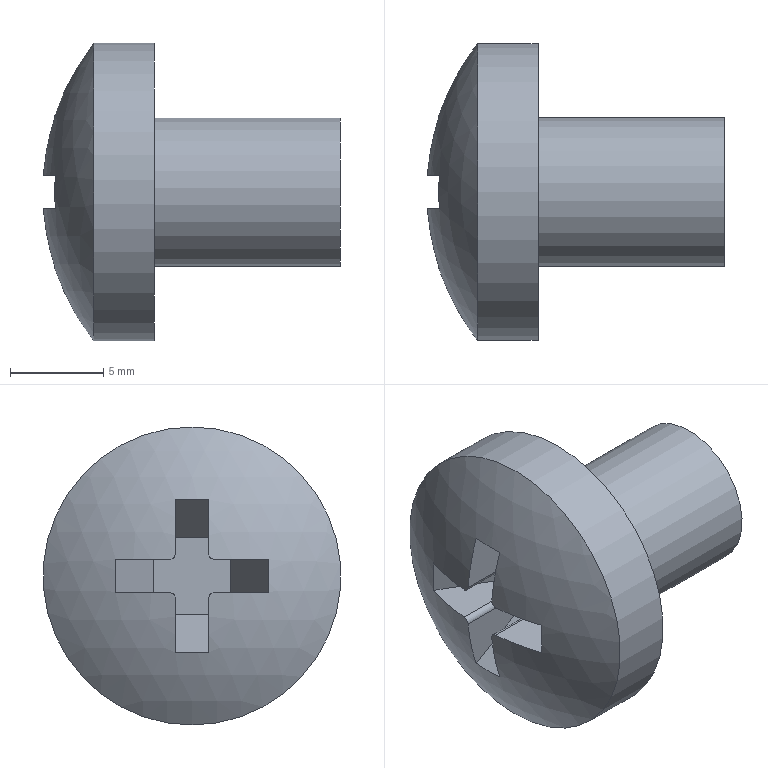Part | STEP file | cross recessed pan head screws gb_GB_CROSS_SCREWS_TYPE1 M8X10-10  H type-N | 1 solid | 22 faces | box 15.925 x 16 x 16 mm | volume 1365 mm3 | plane 15 | cylinder 6 | sphere 1 | commonest cylinder face diameters 0.6 x4 8 x1 16 x1